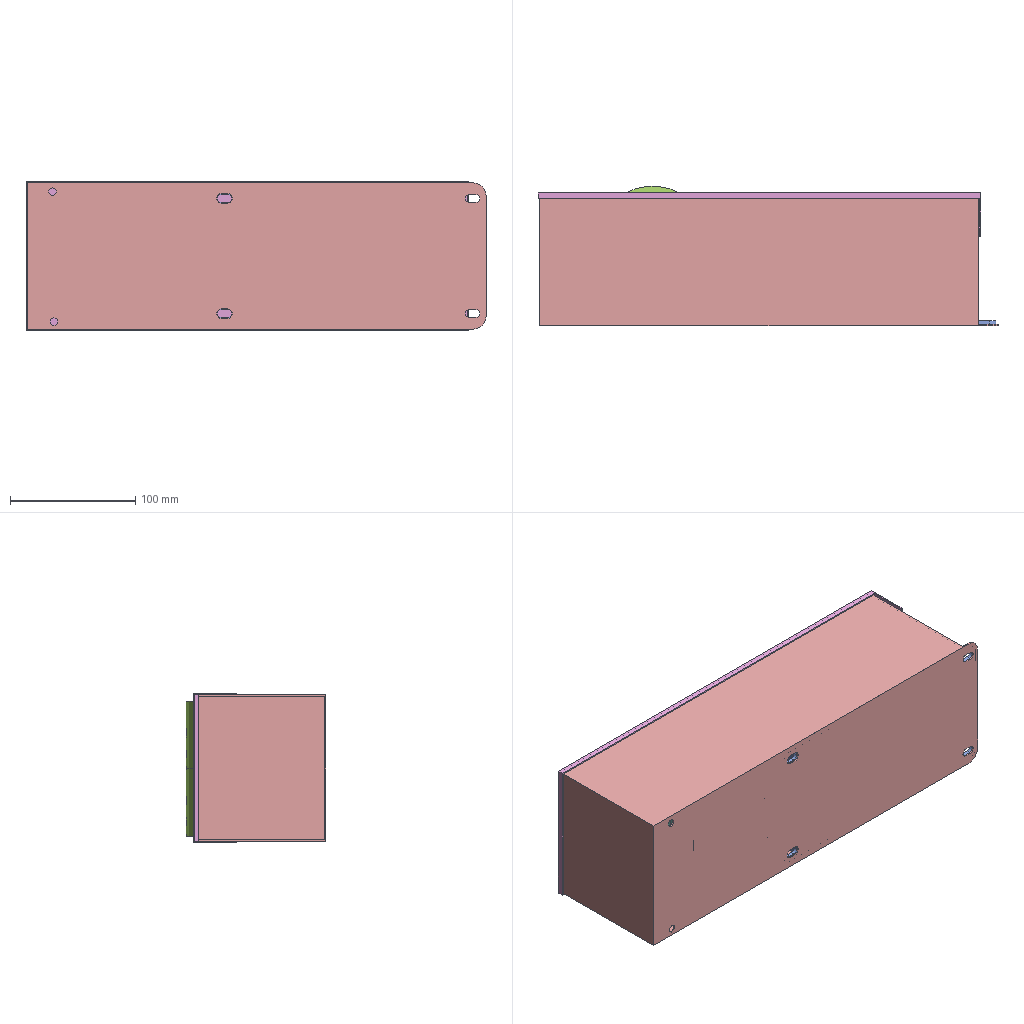Assembly | SolidWorks | 5 different items | 6 placed | box 367 x 111 x 119 mm
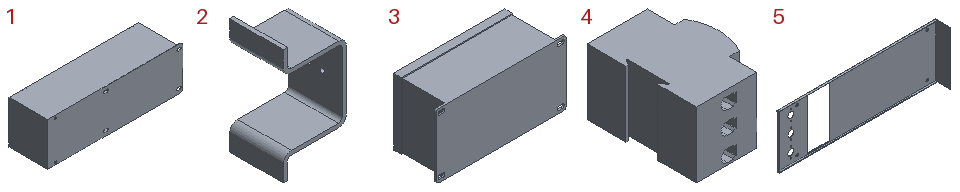Parts list (item | quantity | size | volume | features):
1 | x1 | 366 x 105 x 116.75 mm | 129942 mm3 | features MoveFace 16, ICE 8, Fillet 2, Extrusion 1, HoleWzd 1, Scale 1, Shell 1
2 | x1 | 47 x 40 x 86 mm | 19876 mm3 | features Fillet 2, Extrusion 1, HoleWzd 1, MoveFace 1
3 | x1 | 216 x 86 x 110.411 mm | 1696161 mm3 | features ICE 2, Extrusion 1
4 | x2 | 63.5 x 90 x 54 mm | 247682 mm3 | features ICE 15, MoveFace 7, LPattern 2, Chamfer 1, CombineBodies 1, Extrusion 1, Fillet 1, MirrorPattern 1, PLine 1
5 | x1 | 353.4 x 34.5 x 119.15 mm | 42763 mm3 | features MoveFace 15, ICE 6, Cut 1, Extrusion 1
Mates (type | each side: item.copy, entity, surface, feature):
Coincident | 1.1 face plane Shell1 | 3.1 face plane Boss-Extrude1
Parallel | 1.1 face plane Shell1 | 3.1 face plane Boss-Extrude1
Coincident | 1.1 face plane Boss-Extrude1 | 5.1 face plane Boss-Extrude1 | 2 times
Concentric | 1.1 face cylinder Cut-Extrude1 | 3.1 face cylinder Boss-Extrude1
Coincident | 4.1 face plane Split Line4 | 4.2 face plane LPattern2
Coincident | 4.1 face plane Boss-Extrude1 | 4.2 face plane Boss-Extrude1 | 2 times
Parallel | 1.1 face plane Shell1 | 4.2 face plane Split Line4
DistanceDim | 3.1 face plane Boss-Extrude2 | 4.2 face plane Boss-Extrude1
Coincident | 1.1 face plane Shell1 | 2.1 face plane Boss-Extrude1
Coincident | 4.1 face plane Boss-Extrude1 | 2.1 face plane Boss-Extrude1
DistanceDim | 1.1 face plane Shell1 | 2.1 face plane Boss-Extrude1 | 2 times
DistanceDim | 1.1 face plane Shell1 | 4.1 face plane LPattern2
Concentric | 1.1 face cylinder M4 Tapped Hole1 | 5.1 face cylinder Cut-Extrude1 | 2 times